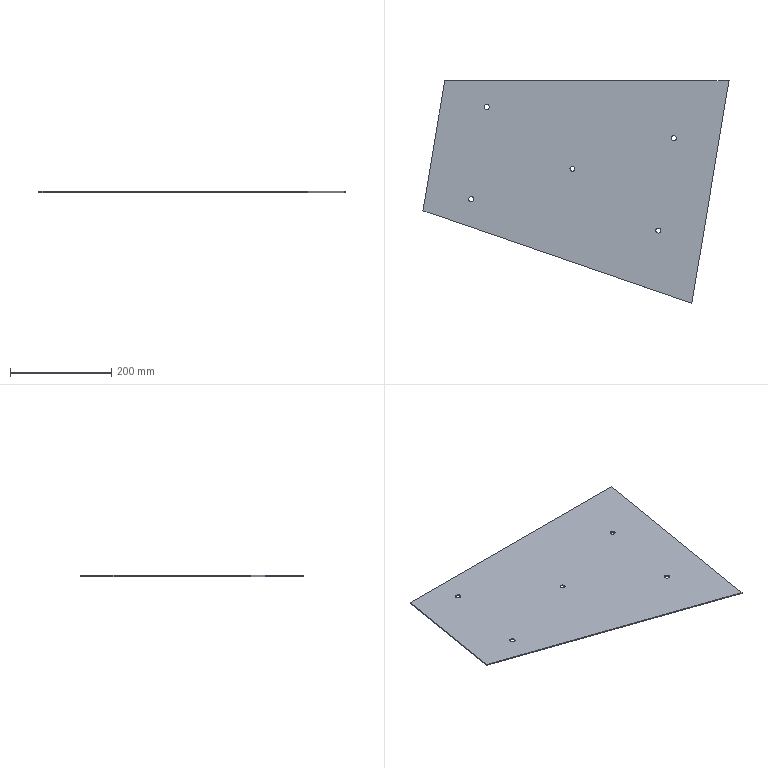Part | SolidWorks | features Extrusion 1, ICE 1 | 1 solid | 16 faces | box 604.658 x 439.557 x 2 mm | volume 390296 mm3 | cylinder 10 | plane 6 | commonest cylinder face diameters 10 x10
STEP:
#1=CARTESIAN_POINT('',(-213.545,-102.176,0.));
#2=VERTEX_POINT('',#1);
#3=CARTESIAN_POINT('',(-203.545,-102.176,0.));
#4=VERTEX_POINT('',#3);
#5=CARTESIAN_POINT('',(-208.545,-102.176,0.));
#6=DIRECTION('',(0.,0.,1.));
#7=DIRECTION('',(1.,0.,0.));
#8=AXIS2_PLACEMENT_3D('',#5,#6,#7);
#9=CIRCLE('',#8,5.);
#10=EDGE_CURVE('',#2,#4,#9,.T.);
#11=ORIENTED_EDGE('',*,*,#10,.F.);
#12=CARTESIAN_POINT('',(-213.545,-102.176,2.));
#13=VERTEX_POINT('',#12);
#14=CARTESIAN_POINT('',(-213.545,-102.176,-8.));
#15=DIRECTION('',(0.,0.,1.));
#16=VECTOR('',#15,1000.);
#17=LINE('',#14,#16);
#18=EDGE_CURVE('',#2,#13,#17,.T.);
#19=ORIENTED_EDGE('',*,*,#18,.T.);
#20=CARTESIAN_POINT('',(-203.545,-102.176,2.));
#21=VERTEX_POINT('',#20);
#22=CARTESIAN_POINT('',(-208.545,-102.176,2.));
#23=DIRECTION('',(0.,0.,1.));
#24=DIRECTION('',(1.,0.,0.));
#25=AXIS2_PLACEMENT_3D('',#22,#23,#24);
#26=CIRCLE('',#25,5.);
#27=EDGE_CURVE('',#13,#21,#26,.T.);
#28=ORIENTED_EDGE('',*,*,#27,.T.);
#29=CARTESIAN_POINT('',(-203.545,-102.176,-8.));
#30=DIRECTION('',(0.,0.,1.));
#31=VECTOR('',#30,1000.);
#32=LINE('',#29,#31);
#33=EDGE_CURVE('',#4,#21,#32,.T.);
#34=ORIENTED_EDGE('',*,*,#33,.F.);
#35=EDGE_LOOP('',(#11,#19,#28,#34));
#36=FACE_OUTER_BOUND('',#35,.T.);
#37=CARTESIAN_POINT('',(-208.545,-102.176,-8.));
#38=DIRECTION('',(0.,0.,1.));
#39=DIRECTION('',(1.,0.,0.));
#40=AXIS2_PLACEMENT_3D('',#37,#38,#39);
#41=CYLINDRICAL_SURFACE('',#40,5.);
#42=ADVANCED_FACE('',(#36),#41,.F.);
#43=CARTESIAN_POINT('',(-244.079,-284.638,0.));
#44=VERTEX_POINT('',#43);
#45=CARTESIAN_POINT('',(-234.079,-284.638,0.));
#46=VERTEX_POINT('',#45);
#47=CARTESIAN_POINT('',(-239.079,-284.638,0.));
#48=DIRECTION('',(0.,0.,1.));
#49=DIRECTION('',(1.,0.,0.));
#50=AXIS2_PLACEMENT_3D('',#47,#48,#49);
#51=CIRCLE('',#50,5.);
#52=EDGE_CURVE('',#44,#46,#51,.T.);
#53=ORIENTED_EDGE('',*,*,#52,.F.);
#54=CARTESIAN_POINT('',(-244.079,-284.638,2.));
#55=VERTEX_POINT('',#54);
#56=CARTESIAN_POINT('',(-244.079,-284.638,-8.));
#57=DIRECTION('',(0.,0.,1.));
#58=VECTOR('',#57,1000.);
#59=LINE('',#56,#58);
#60=EDGE_CURVE('',#44,#55,#59,.T.);
#61=ORIENTED_EDGE('',*,*,#60,.T.);
#62=CARTESIAN_POINT('',(-234.079,-284.638,2.));
#63=VERTEX_POINT('',#62);
#64=CARTESIAN_POINT('',(-239.079,-284.638,2.));
#65=DIRECTION('',(0.,0.,1.));
#66=DIRECTION('',(1.,0.,0.));
#67=AXIS2_PLACEMENT_3D('',#64,#65,#66);
#68=CIRCLE('',#67,5.);
#69=EDGE_CURVE('',#55,#63,#68,.T.);
#70=ORIENTED_EDGE('',*,*,#69,.T.);
#71=CARTESIAN_POINT('',(-234.079,-284.638,-8.));
#72=DIRECTION('',(0.,0.,1.));
#73=VECTOR('',#72,1000.);
#74=LINE('',#71,#73);
#75=EDGE_CURVE('',#46,#63,#74,.T.);
#76=ORIENTED_EDGE('',*,*,#75,.F.);
#77=EDGE_LOOP('',(#53,#61,#70,#76));
#78=FACE_OUTER_BOUND('',#77,.T.);
#79=CARTESIAN_POINT('',(-239.079,-284.638,-8.));
#80=DIRECTION('',(0.,0.,1.));
#81=DIRECTION('',(1.,0.,0.));
#82=AXIS2_PLACEMENT_3D('',#79,#80,#81);
#83=CYLINDRICAL_SURFACE('',#82,5.);
#84=ADVANCED_FACE('',(#78),#83,.F.);
#85=CARTESIAN_POINT('',(-43.884,-224.353,0.));
#86=VERTEX_POINT('',#85);
#87=CARTESIAN_POINT('',(-33.884,-224.353,0.));
#88=VERTEX_POINT('',#87);
#89=CARTESIAN_POINT('',(-38.884,-224.353,0.));
#90=DIRECTION('',(0.,0.,1.));
#91=DIRECTION('',(1.,0.,0.));
#92=AXIS2_PLACEMENT_3D('',#89,#90,#91);
#93=CIRCLE('',#92,5.);
#94=EDGE_CURVE('',#86,#88,#93,.T.);
#95=ORIENTED_EDGE('',*,*,#94,.F.);
#96=CARTESIAN_POINT('',(-43.884,-224.353,2.));
#97=VERTEX_POINT('',#96);
#98=CARTESIAN_POINT('',(-43.884,-224.353,-8.));
#99=DIRECTION('',(0.,0.,1.));
#100=VECTOR('',#99,1000.);
#101=LINE('',#98,#100);
#102=EDGE_CURVE('',#86,#97,#101,.T.);
#103=ORIENTED_EDGE('',*,*,#102,.T.);
#104=CARTESIAN_POINT('',(-33.884,-224.353,2.));
#105=VERTEX_POINT('',#104);
#106=CARTESIAN_POINT('',(-38.884,-224.353,2.));
#107=DIRECTION('',(0.,0.,1.));
#108=DIRECTION('',(1.,0.,0.));
#109=AXIS2_PLACEMENT_3D('',#106,#107,#108);
#110=CIRCLE('',#109,5.);
#111=EDGE_CURVE('',#97,#105,#110,.T.);
#112=ORIENTED_EDGE('',*,*,#111,.T.);
#113=CARTESIAN_POINT('',(-33.884,-224.353,-8.));
#114=DIRECTION('',(0.,0.,1.));
#115=VECTOR('',#114,1000.);
#116=LINE('',#113,#115);
#117=EDGE_CURVE('',#88,#105,#116,.T.);
#118=ORIENTED_EDGE('',*,*,#117,.F.);
#119=EDGE_LOOP('',(#95,#103,#112,#118));
#120=FACE_OUTER_BOUND('',#119,.T.);
#121=CARTESIAN_POINT('',(-38.884,-224.353,-8.));
#122=DIRECTION('',(0.,0.,1.));
#123=DIRECTION('',(1.,0.,0.));
#124=AXIS2_PLACEMENT_3D('',#121,#122,#123);
#125=CYLINDRICAL_SURFACE('',#124,5.);
#126=ADVANCED_FACE('',(#120),#125,.F.);
#127=CARTESIAN_POINT('',(125.778,-346.531,0.));
#128=VERTEX_POINT('',#127);
#129=CARTESIAN_POINT('',(135.778,-346.531,0.));
#130=VERTEX_POINT('',#129);
#131=CARTESIAN_POINT('',(130.778,-346.531,0.));
#132=DIRECTION('',(0.,0.,1.));
#133=DIRECTION('',(1.,0.,0.));
#134=AXIS2_PLACEMENT_3D('',#131,#132,#133);
#135=CIRCLE('',#134,5.);
#136=EDGE_CURVE('',#128,#130,#135,.T.);
#137=ORIENTED_EDGE('',*,*,#136,.F.);
#138=CARTESIAN_POINT('',(125.778,-346.531,2.));
#139=VERTEX_POINT('',#138);
#140=CARTESIAN_POINT('',(125.778,-346.531,-8.));
#141=DIRECTION('',(0.,0.,1.));
#142=VECTOR('',#141,1000.);
#143=LINE('',#140,#142);
#144=EDGE_CURVE('',#128,#139,#143,.T.);
#145=ORIENTED_EDGE('',*,*,#144,.T.);
#146=CARTESIAN_POINT('',(135.778,-346.531,2.));
#147=VERTEX_POINT('',#146);
#148=CARTESIAN_POINT('',(130.778,-346.531,2.));
#149=DIRECTION('',(0.,0.,1.));
#150=DIRECTION('',(1.,0.,0.));
#151=AXIS2_PLACEMENT_3D('',#148,#149,#150);
#152=CIRCLE('',#151,5.);
#153=EDGE_CURVE('',#139,#147,#152,.T.);
#154=ORIENTED_EDGE('',*,*,#153,.T.);
#155=CARTESIAN_POINT('',(135.778,-346.531,-8.));
#156=DIRECTION('',(0.,0.,1.));
#157=VECTOR('',#156,1000.);
#158=LINE('',#155,#157);
#159=EDGE_CURVE('',#130,#147,#158,.T.);
#160=ORIENTED_EDGE('',*,*,#159,.F.);
#161=EDGE_LOOP('',(#137,#145,#154,#160));
#162=FACE_OUTER_BOUND('',#161,.T.);
#163=CARTESIAN_POINT('',(130.778,-346.531,-8.));
#164=DIRECTION('',(0.,0.,1.));
#165=DIRECTION('',(1.,0.,0.));
#166=AXIS2_PLACEMENT_3D('',#163,#164,#165);
#167=CYLINDRICAL_SURFACE('',#166,5.);
#168=ADVANCED_FACE('',(#162),#167,.F.);
#169=CARTESIAN_POINT('',(156.312,-164.068,0.));
#170=VERTEX_POINT('',#169);
#171=CARTESIAN_POINT('',(166.312,-164.068,0.));
#172=VERTEX_POINT('',#171);
#173=CARTESIAN_POINT('',(161.312,-164.068,0.));
#174=DIRECTION('',(0.,0.,1.));
#175=DIRECTION('',(1.,0.,0.));
#176=AXIS2_PLACEMENT_3D('',#173,#174,#175);
#177=CIRCLE('',#176,5.);
#178=EDGE_CURVE('',#170,#172,#177,.T.);
#179=ORIENTED_EDGE('',*,*,#178,.F.);
#180=CARTESIAN_POINT('',(156.312,-164.068,2.));
#181=VERTEX_POINT('',#180);
#182=CARTESIAN_POINT('',(156.312,-164.068,-8.));
#183=DIRECTION('',(0.,0.,1.));
#184=VECTOR('',#183,1000.);
#185=LINE('',#182,#184);
#186=EDGE_CURVE('',#170,#181,#185,.T.);
#187=ORIENTED_EDGE('',*,*,#186,.T.);
#188=CARTESIAN_POINT('',(166.312,-164.068,2.));
#189=VERTEX_POINT('',#188);
#190=CARTESIAN_POINT('',(161.312,-164.068,2.));
#191=DIRECTION('',(0.,0.,1.));
#192=DIRECTION('',(1.,0.,0.));
#193=AXIS2_PLACEMENT_3D('',#190,#191,#192);
#194=CIRCLE('',#193,5.);
#195=EDGE_CURVE('',#181,#189,#194,.T.);
#196=ORIENTED_EDGE('',*,*,#195,.T.);
#197=CARTESIAN_POINT('',(166.312,-164.068,-8.));
#198=DIRECTION('',(0.,0.,1.));
#199=VECTOR('',#198,1000.);
#200=LINE('',#197,#199);
#201=EDGE_CURVE('',#172,#189,#200,.T.);
#202=ORIENTED_EDGE('',*,*,#201,.F.);
#203=EDGE_LOOP('',(#179,#187,#196,#202));
#204=FACE_OUTER_BOUND('',#203,.T.);
#205=CARTESIAN_POINT('',(161.312,-164.068,-8.));
#206=DIRECTION('',(0.,0.,1.));
#207=DIRECTION('',(1.,0.,0.));
#208=AXIS2_PLACEMENT_3D('',#205,#206,#207);
#209=CYLINDRICAL_SURFACE('',#208,5.);
#210=ADVANCED_FACE('',(#204),#209,.F.);
#211=CARTESIAN_POINT('',(196.87,-490.036,0.));
#212=VERTEX_POINT('',#211);
#213=CARTESIAN_POINT('',(270.426,-50.479,0.));
#214=VERTEX_POINT('',#213);
#215=CARTESIAN_POINT('',(196.87,-490.036,0.));
#216=DIRECTION('',(0.165,0.9863,0.));
#217=VECTOR('',#216,1000.);
#218=LINE('',#215,#217);
#219=EDGE_CURVE('',#212,#214,#218,.T.);
#220=ORIENTED_EDGE('',*,*,#219,.T.);
#221=CARTESIAN_POINT('',(270.426,-50.479,2.));
#222=VERTEX_POINT('',#221);
#223=CARTESIAN_POINT('',(270.426,-50.479,2.));
#224=DIRECTION('',(0.,0.,-1.));
#225=VECTOR('',#224,1000.);
#226=LINE('',#223,#225);
#227=EDGE_CURVE('',#222,#214,#226,.T.);
#228=ORIENTED_EDGE('',*,*,#227,.F.);
#229=CARTESIAN_POINT('',(196.87,-490.036,2.));
#230=VERTEX_POINT('',#229);
#231=CARTESIAN_POINT('',(196.87,-490.036,2.));
#232=DIRECTION('',(0.165,0.9863,0.));
#233=VECTOR('',#232,1000.);
#234=LINE('',#231,#233);
#235=EDGE_CURVE('',#230,#222,#234,.T.);
#236=ORIENTED_EDGE('',*,*,#235,.F.);
#237=CARTESIAN_POINT('',(196.87,-490.036,2.));
#238=DIRECTION('',(0.,0.,-1.));
#239=VECTOR('',#238,1000.);
#240=LINE('',#237,#239);
#241=EDGE_CURVE('',#230,#212,#240,.T.);
#242=ORIENTED_EDGE('',*,*,#241,.T.);
#243=EDGE_LOOP('',(#220,#228,#236,#242));
#244=FACE_OUTER_BOUND('',#243,.T.);
#245=CARTESIAN_POINT('',(196.87,-490.036,2.));
#246=DIRECTION('',(-0.9863,0.165,0.));
#247=DIRECTION('',(-0.165,-0.9863,0.));
#248=AXIS2_PLACEMENT_3D('',#245,#246,#247);
#249=PLANE('',#248);
#250=ADVANCED_FACE('',(#244),#249,.F.);
#251=CARTESIAN_POINT('',(-291.277,-50.479,0.));
#252=VERTEX_POINT('',#251);
#253=CARTESIAN_POINT('',(270.426,-50.479,0.));
#254=DIRECTION('',(-1.,0.,0.));
#255=VECTOR('',#254,1000.);
#256=LINE('',#253,#255);
#257=EDGE_CURVE('',#214,#252,#256,.T.);
#258=ORIENTED_EDGE('',*,*,#257,.T.);
#259=CARTESIAN_POINT('',(-291.277,-50.479,2.));
#260=VERTEX_POINT('',#259);
#261=CARTESIAN_POINT('',(-291.277,-50.479,2.));
#262=DIRECTION('',(0.,0.,-1.));
#263=VECTOR('',#262,1000.);
#264=LINE('',#261,#263);
#265=EDGE_CURVE('',#260,#252,#264,.T.);
#266=ORIENTED_EDGE('',*,*,#265,.F.);
#267=CARTESIAN_POINT('',(270.426,-50.479,2.));
#268=DIRECTION('',(-1.,0.,0.));
#269=VECTOR('',#268,1000.);
#270=LINE('',#267,#269);
#271=EDGE_CURVE('',#222,#260,#270,.T.);
#272=ORIENTED_EDGE('',*,*,#271,.F.);
#273=ORIENTED_EDGE('',*,*,#227,.T.);
#274=EDGE_LOOP('',(#258,#266,#272,#273));
#275=FACE_OUTER_BOUND('',#274,.T.);
#276=CARTESIAN_POINT('',(270.426,-50.479,2.));
#277=DIRECTION('',(0.,-1.,0.));
#278=DIRECTION('',(1.,0.,0.));
#279=AXIS2_PLACEMENT_3D('',#276,#277,#278);
#280=PLANE('',#279);
#281=ADVANCED_FACE('',(#275),#280,.F.);
#282=CARTESIAN_POINT('',(-334.231,-307.164,0.));
#283=VERTEX_POINT('',#282);
#284=CARTESIAN_POINT('',(-291.277,-50.479,0.));
#285=DIRECTION('',(-0.165,-0.9863,0.));
#286=VECTOR('',#285,1000.);
#287=LINE('',#284,#286);
#288=EDGE_CURVE('',#252,#283,#287,.T.);
#289=ORIENTED_EDGE('',*,*,#288,.T.);
#290=CARTESIAN_POINT('',(-334.231,-307.164,2.));
#291=VERTEX_POINT('',#290);
#292=CARTESIAN_POINT('',(-334.231,-307.164,2.));
#293=DIRECTION('',(0.,0.,-1.));
#294=VECTOR('',#293,1000.);
#295=LINE('',#292,#294);
#296=EDGE_CURVE('',#291,#283,#295,.T.);
#297=ORIENTED_EDGE('',*,*,#296,.F.);
#298=CARTESIAN_POINT('',(-291.277,-50.479,2.));
#299=DIRECTION('',(-0.165,-0.9863,0.));
#300=VECTOR('',#299,1000.);
#301=LINE('',#298,#300);
#302=EDGE_CURVE('',#260,#291,#301,.T.);
#303=ORIENTED_EDGE('',*,*,#302,.F.);
#304=ORIENTED_EDGE('',*,*,#265,.T.);
#305=EDGE_LOOP('',(#289,#297,#303,#304));
#306=FACE_OUTER_BOUND('',#305,.T.);
#307=CARTESIAN_POINT('',(-291.277,-50.479,2.));
#308=DIRECTION('',(0.9863,-0.165,0.));
#309=DIRECTION('',(0.165,0.9863,0.));
#310=AXIS2_PLACEMENT_3D('',#307,#308,#309);
#311=PLANE('',#310);
#312=ADVANCED_FACE('',(#306),#311,.F.);
#313=CARTESIAN_POINT('',(-334.231,-307.164,0.));
#314=DIRECTION('',(0.9455,-0.3256,0.));
#315=VECTOR('',#314,1000.);
#316=LINE('',#313,#315);
#317=EDGE_CURVE('',#283,#212,#316,.T.);
#318=ORIENTED_EDGE('',*,*,#317,.T.);
#319=ORIENTED_EDGE('',*,*,#241,.F.);
#320=CARTESIAN_POINT('',(-334.231,-307.164,2.));
#321=DIRECTION('',(0.9455,-0.3256,0.));
#322=VECTOR('',#321,1000.);
#323=LINE('',#320,#322);
#324=EDGE_CURVE('',#291,#230,#323,.T.);
#325=ORIENTED_EDGE('',*,*,#324,.F.);
#326=ORIENTED_EDGE('',*,*,#296,.T.);
#327=EDGE_LOOP('',(#318,#319,#325,#326));
#328=FACE_OUTER_BOUND('',#327,.T.);
#329=CARTESIAN_POINT('',(-334.231,-307.164,2.));
#330=DIRECTION('',(0.3256,0.9455,0.));
#331=DIRECTION('',(-0.9455,0.3256,0.));
#332=AXIS2_PLACEMENT_3D('',#329,#330,#331);
#333=PLANE('',#332);
#334=ADVANCED_FACE('',(#328),#333,.F.);
#335=CARTESIAN_POINT('',(-208.545,-102.176,2.));
#336=DIRECTION('',(0.,0.,1.));
#337=DIRECTION('',(1.,0.,0.));
#338=AXIS2_PLACEMENT_3D('',#335,#336,#337);
#339=CIRCLE('',#338,5.);
#340=EDGE_CURVE('',#21,#13,#339,.T.);
#341=ORIENTED_EDGE('',*,*,#340,.F.);
#342=ORIENTED_EDGE('',*,*,#27,.F.);
#343=EDGE_LOOP('',(#341,#342));
#344=FACE_BOUND('',#343,.T.);
#345=CARTESIAN_POINT('',(-239.079,-284.638,2.));
#346=DIRECTION('',(0.,0.,1.));
#347=DIRECTION('',(1.,0.,0.));
#348=AXIS2_PLACEMENT_3D('',#345,#346,#347);
#349=CIRCLE('',#348,5.);
#350=EDGE_CURVE('',#63,#55,#349,.T.);
#351=ORIENTED_EDGE('',*,*,#350,.F.);
#352=ORIENTED_EDGE('',*,*,#69,.F.);
#353=EDGE_LOOP('',(#351,#352));
#354=FACE_BOUND('',#353,.T.);
#355=CARTESIAN_POINT('',(-38.884,-224.353,2.));
#356=DIRECTION('',(0.,0.,1.));
#357=DIRECTION('',(1.,0.,0.));
#358=AXIS2_PLACEMENT_3D('',#355,#356,#357);
#359=CIRCLE('',#358,5.);
#360=EDGE_CURVE('',#105,#97,#359,.T.);
#361=ORIENTED_EDGE('',*,*,#360,.F.);
#362=ORIENTED_EDGE('',*,*,#111,.F.);
#363=EDGE_LOOP('',(#361,#362));
#364=FACE_BOUND('',#363,.T.);
#365=CARTESIAN_POINT('',(130.778,-346.531,2.));
#366=DIRECTION('',(0.,0.,1.));
#367=DIRECTION('',(1.,0.,0.));
#368=AXIS2_PLACEMENT_3D('',#365,#366,#367);
#369=CIRCLE('',#368,5.);
#370=EDGE_CURVE('',#147,#139,#369,.T.);
#371=ORIENTED_EDGE('',*,*,#370,.F.);
#372=ORIENTED_EDGE('',*,*,#153,.F.);
#373=EDGE_LOOP('',(#371,#372));
#374=FACE_BOUND('',#373,.T.);
#375=CARTESIAN_POINT('',(161.312,-164.068,2.));
#376=DIRECTION('',(0.,0.,1.));
#377=DIRECTION('',(1.,0.,0.));
#378=AXIS2_PLACEMENT_3D('',#375,#376,#377);
#379=CIRCLE('',#378,5.);
#380=EDGE_CURVE('',#189,#181,#379,.T.);
#381=ORIENTED_EDGE('',*,*,#380,.F.);
#382=ORIENTED_EDGE('',*,*,#195,.F.);
#383=EDGE_LOOP('',(#381,#382));
#384=FACE_BOUND('',#383,.T.);
#385=ORIENTED_EDGE('',*,*,#235,.T.);
#386=ORIENTED_EDGE('',*,*,#271,.T.);
#387=ORIENTED_EDGE('',*,*,#302,.T.);
#388=ORIENTED_EDGE('',*,*,#324,.T.);
#389=EDGE_LOOP('',(#385,#386,#387,#388));
#390=FACE_OUTER_BOUND('',#389,.T.);
#391=CARTESIAN_POINT('',(0.,0.,2.));
#392=DIRECTION('',(0.,0.,1.));
#393=DIRECTION('',(1.,0.,0.));
#394=AXIS2_PLACEMENT_3D('',#391,#392,#393);
#395=PLANE('',#394);
#396=ADVANCED_FACE('',(#344,#354,#364,#374,#384,#390),#395,.T.);
#397=CARTESIAN_POINT('',(-208.545,-102.176,0.));
#398=DIRECTION('',(0.,0.,1.));
#399=DIRECTION('',(1.,0.,0.));
#400=AXIS2_PLACEMENT_3D('',#397,#398,#399);
#401=CIRCLE('',#400,5.);
#402=EDGE_CURVE('',#4,#2,#401,.T.);
#403=ORIENTED_EDGE('',*,*,#402,.T.);
#404=ORIENTED_EDGE('',*,*,#10,.T.);
#405=EDGE_LOOP('',(#403,#404));
#406=FACE_BOUND('',#405,.T.);
#407=CARTESIAN_POINT('',(-239.079,-284.638,0.));
#408=DIRECTION('',(0.,0.,1.));
#409=DIRECTION('',(1.,0.,0.));
#410=AXIS2_PLACEMENT_3D('',#407,#408,#409);
#411=CIRCLE('',#410,5.);
#412=EDGE_CURVE('',#46,#44,#411,.T.);
#413=ORIENTED_EDGE('',*,*,#412,.T.);
#414=ORIENTED_EDGE('',*,*,#52,.T.);
#415=EDGE_LOOP('',(#413,#414));
#416=FACE_BOUND('',#415,.T.);
#417=CARTESIAN_POINT('',(-38.884,-224.353,0.));
#418=DIRECTION('',(0.,0.,1.));
#419=DIRECTION('',(1.,0.,0.));
#420=AXIS2_PLACEMENT_3D('',#417,#418,#419);
#421=CIRCLE('',#420,5.);
#422=EDGE_CURVE('',#88,#86,#421,.T.);
#423=ORIENTED_EDGE('',*,*,#422,.T.);
#424=ORIENTED_EDGE('',*,*,#94,.T.);
#425=EDGE_LOOP('',(#423,#424));
#426=FACE_BOUND('',#425,.T.);
#427=CARTESIAN_POINT('',(130.778,-346.531,0.));
#428=DIRECTION('',(0.,0.,1.));
#429=DIRECTION('',(1.,0.,0.));
#430=AXIS2_PLACEMENT_3D('',#427,#428,#429);
#431=CIRCLE('',#430,5.);
#432=EDGE_CURVE('',#130,#128,#431,.T.);
#433=ORIENTED_EDGE('',*,*,#432,.T.);
#434=ORIENTED_EDGE('',*,*,#136,.T.);
#435=EDGE_LOOP('',(#433,#434));
#436=FACE_BOUND('',#435,.T.);
#437=CARTESIAN_POINT('',(161.312,-164.068,0.));
#438=DIRECTION('',(0.,0.,1.));
#439=DIRECTION('',(1.,0.,0.));
#440=AXIS2_PLACEMENT_3D('',#437,#438,#439);
#441=CIRCLE('',#440,5.);
#442=EDGE_CURVE('',#172,#170,#441,.T.);
#443=ORIENTED_EDGE('',*,*,#442,.T.);
#444=ORIENTED_EDGE('',*,*,#178,.T.);
#445=EDGE_LOOP('',(#443,#444));
#446=FACE_BOUND('',#445,.T.);
#447=ORIENTED_EDGE('',*,*,#219,.F.);
#448=ORIENTED_EDGE('',*,*,#317,.F.);
#449=ORIENTED_EDGE('',*,*,#288,.F.);
#450=ORIENTED_EDGE('',*,*,#257,.F.);
#451=EDGE_LOOP('',(#447,#448,#449,#450));
#452=FACE_OUTER_BOUND('',#451,.T.);
#453=CARTESIAN_POINT('',(0.,0.,0.));
#454=DIRECTION('',(0.,0.,1.));
#455=DIRECTION('',(1.,0.,0.));
#456=AXIS2_PLACEMENT_3D('',#453,#454,#455);
#457=PLANE('',#456);
#458=ADVANCED_FACE('',(#406,#416,#426,#436,#446,#452),#457,.F.);
#459=ORIENTED_EDGE('',*,*,#186,.F.);
#460=ORIENTED_EDGE('',*,*,#442,.F.);
#461=ORIENTED_EDGE('',*,*,#201,.T.);
#462=ORIENTED_EDGE('',*,*,#380,.T.);
#463=EDGE_LOOP('',(#459,#460,#461,#462));
#464=FACE_OUTER_BOUND('',#463,.T.);
#465=CARTESIAN_POINT('',(161.312,-164.068,-8.));
#466=DIRECTION('',(0.,0.,1.));
#467=DIRECTION('',(1.,0.,0.));
#468=AXIS2_PLACEMENT_3D('',#465,#466,#467);
#469=CYLINDRICAL_SURFACE('',#468,5.);
#470=ADVANCED_FACE('',(#464),#469,.F.);
#471=ORIENTED_EDGE('',*,*,#144,.F.);
#472=ORIENTED_EDGE('',*,*,#432,.F.);
#473=ORIENTED_EDGE('',*,*,#159,.T.);
#474=ORIENTED_EDGE('',*,*,#370,.T.);
#475=EDGE_LOOP('',(#471,#472,#473,#474));
#476=FACE_OUTER_BOUND('',#475,.T.);
#477=CARTESIAN_POINT('',(130.778,-346.531,-8.));
#478=DIRECTION('',(0.,0.,1.));
#479=DIRECTION('',(1.,0.,0.));
#480=AXIS2_PLACEMENT_3D('',#477,#478,#479);
#481=CYLINDRICAL_SURFACE('',#480,5.);
#482=ADVANCED_FACE('',(#476),#481,.F.);
#483=ORIENTED_EDGE('',*,*,#102,.F.);
#484=ORIENTED_EDGE('',*,*,#422,.F.);
#485=ORIENTED_EDGE('',*,*,#117,.T.);
#486=ORIENTED_EDGE('',*,*,#360,.T.);
#487=EDGE_LOOP('',(#483,#484,#485,#486));
#488=FACE_OUTER_BOUND('',#487,.T.);
#489=CARTESIAN_POINT('',(-38.884,-224.353,-8.));
#490=DIRECTION('',(0.,0.,1.));
#491=DIRECTION('',(1.,0.,0.));
#492=AXIS2_PLACEMENT_3D('',#489,#490,#491);
#493=CYLINDRICAL_SURFACE('',#492,5.);
#494=ADVANCED_FACE('',(#488),#493,.F.);
#495=ORIENTED_EDGE('',*,*,#60,.F.);
#496=ORIENTED_EDGE('',*,*,#412,.F.);
#497=ORIENTED_EDGE('',*,*,#75,.T.);
#498=ORIENTED_EDGE('',*,*,#350,.T.);
#499=EDGE_LOOP('',(#495,#496,#497,#498));
#500=FACE_OUTER_BOUND('',#499,.T.);
#501=CARTESIAN_POINT('',(-239.079,-284.638,-8.));
#502=DIRECTION('',(0.,0.,1.));
#503=DIRECTION('',(1.,0.,0.));
#504=AXIS2_PLACEMENT_3D('',#501,#502,#503);
#505=CYLINDRICAL_SURFACE('',#504,5.);
#506=ADVANCED_FACE('',(#500),#505,.F.);
#507=ORIENTED_EDGE('',*,*,#18,.F.);
#508=ORIENTED_EDGE('',*,*,#402,.F.);
#509=ORIENTED_EDGE('',*,*,#33,.T.);
#510=ORIENTED_EDGE('',*,*,#340,.T.);
#511=EDGE_LOOP('',(#507,#508,#509,#510));
#512=FACE_OUTER_BOUND('',#511,.T.);
#513=CARTESIAN_POINT('',(-208.545,-102.176,-8.));
#514=DIRECTION('',(0.,0.,1.));
#515=DIRECTION('',(1.,0.,0.));
#516=AXIS2_PLACEMENT_3D('',#513,#514,#515);
#517=CYLINDRICAL_SURFACE('',#516,5.);
#518=ADVANCED_FACE('',(#512),#517,.F.);
#519=CLOSED_SHELL('',(#42,#84,#126,#168,#210,#250,#281,#312,#334,#396,#458,#470,#482,#494,#506,#518));
#520=MANIFOLD_SOLID_BREP('',#519);
#521=CARTESIAN_POINT('',(0.,0.,0.));
#522=DIRECTION('',(0.,0.,1.));
#523=DIRECTION('',(1.,0.,0.));
#524=AXIS2_PLACEMENT_3D('',#521,#522,#523);
#525=(LENGTH_UNIT()NAMED_UNIT(*)SI_UNIT(.MILLI.,.METRE.));
#526=UNCERTAINTY_MEASURE_WITH_UNIT(LENGTH_MEASURE(0.00001),#525,'','');
#527=(NAMED_UNIT(*)PLANE_ANGLE_UNIT()SI_UNIT($,.RADIAN.));
#528=(NAMED_UNIT(*)SI_UNIT($,.STERADIAN.)SOLID_ANGLE_UNIT());
#529=(GEOMETRIC_REPRESENTATION_CONTEXT(3)GLOBAL_UNCERTAINTY_ASSIGNED_CONTEXT((#526))GLOBAL_UNIT_ASSIGNED_CONTEXT((#525,#527,#528))REPRESENTATION_CONTEXT('',''));
#530=ADVANCED_BREP_SHAPE_REPRESENTATION('',(#520,#524),#529);